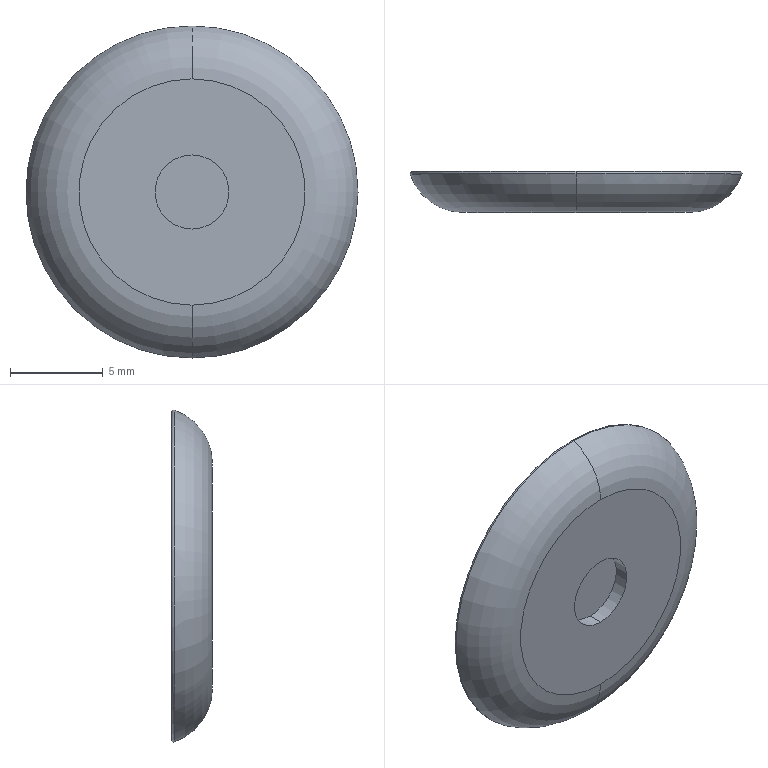Part | SolidWorks | features Revolution 1 | 1 solid | 23 faces | box 17.931 x 2.2 x 17.931 mm | volume 454.739 mm3 | torus 12 | cylinder 6 | plane 5 | commonest cylinder face diameters 4 x2 15.9 x2 16.5 x2
STEP:
#1=CARTESIAN_POINT('',(0.,1.669,-8.961));
#2=VERTEX_POINT('',#1);
#3=CARTESIAN_POINT('',(0.,1.669,8.961));
#4=VERTEX_POINT('',#3);
#5=CARTESIAN_POINT('',(0.,1.669,0.));
#6=DIRECTION('',(0.,-1.,0.));
#7=DIRECTION('',(0.,0.,-1.));
#8=AXIS2_PLACEMENT_3D('',#5,#6,#7);
#9=CIRCLE('',#8,8.961);
#10=EDGE_CURVE('',#2,#4,#9,.T.);
#11=ORIENTED_EDGE('',*,*,#10,.T.);
#12=CARTESIAN_POINT('',(0.,-0.4,6.109));
#13=VERTEX_POINT('',#12);
#14=CARTESIAN_POINT('',(0.,2.6,6.109));
#15=DIRECTION('',(1.,0.,0.));
#16=DIRECTION('',(0.,0.,-1.));
#17=AXIS2_PLACEMENT_3D('',#14,#15,#16);
#18=CIRCLE('',#17,3.);
#19=EDGE_CURVE('',#4,#13,#18,.T.);
#20=ORIENTED_EDGE('',*,*,#19,.T.);
#21=CARTESIAN_POINT('',(0.,-0.4,-6.109));
#22=VERTEX_POINT('',#21);
#23=CARTESIAN_POINT('',(0.,-0.4,0.));
#24=DIRECTION('',(0.,-1.,0.));
#25=DIRECTION('',(0.,0.,-1.));
#26=AXIS2_PLACEMENT_3D('',#23,#24,#25);
#27=CIRCLE('',#26,6.109);
#28=EDGE_CURVE('',#22,#13,#27,.T.);
#29=ORIENTED_EDGE('',*,*,#28,.F.);
#30=CARTESIAN_POINT('',(0.,2.6,-6.109));
#31=DIRECTION('',(-1.,0.,0.));
#32=DIRECTION('',(0.,0.,1.));
#33=AXIS2_PLACEMENT_3D('',#30,#31,#32);
#34=CIRCLE('',#33,3.);
#35=EDGE_CURVE('',#2,#22,#34,.T.);
#36=ORIENTED_EDGE('',*,*,#35,.F.);
#37=EDGE_LOOP('',(#11,#20,#29,#36));
#38=FACE_OUTER_BOUND('',#37,.T.);
#39=CARTESIAN_POINT('',(0.,2.6,0.));
#40=DIRECTION('',(0.,-1.,0.));
#41=DIRECTION('',(0.,0.,-1.));
#42=AXIS2_PLACEMENT_3D('',#39,#40,#41);
#43=TOROIDAL_SURFACE('',#42,6.109,3.);
#44=ADVANCED_FACE('',(#38),#43,.T.);
#45=CARTESIAN_POINT('',(0.,0.4,2.));
#46=VERTEX_POINT('',#45);
#47=CARTESIAN_POINT('',(0.,0.4,-2.));
#48=VERTEX_POINT('',#47);
#49=CARTESIAN_POINT('',(0.,0.4,0.));
#50=DIRECTION('',(0.,-1.,0.));
#51=DIRECTION('',(0.,0.,-1.));
#52=AXIS2_PLACEMENT_3D('',#49,#50,#51);
#53=CIRCLE('',#52,2.);
#54=EDGE_CURVE('',#46,#48,#53,.T.);
#55=ORIENTED_EDGE('',*,*,#54,.F.);
#56=CARTESIAN_POINT('',(0.,-0.4,2.));
#57=VERTEX_POINT('',#56);
#58=CARTESIAN_POINT('',(0.,0.,2.));
#59=DIRECTION('',(0.,-1.,0.));
#60=VECTOR('',#59,1000.);
#61=LINE('',#58,#60);
#62=EDGE_CURVE('',#46,#57,#61,.T.);
#63=ORIENTED_EDGE('',*,*,#62,.T.);
#64=CARTESIAN_POINT('',(0.,-0.4,-2.));
#65=VERTEX_POINT('',#64);
#66=CARTESIAN_POINT('',(0.,-0.4,0.));
#67=DIRECTION('',(0.,-1.,0.));
#68=DIRECTION('',(0.,0.,-1.));
#69=AXIS2_PLACEMENT_3D('',#66,#67,#68);
#70=CIRCLE('',#69,2.);
#71=EDGE_CURVE('',#57,#65,#70,.T.);
#72=ORIENTED_EDGE('',*,*,#71,.T.);
#73=CARTESIAN_POINT('',(0.,0.,-2.));
#74=DIRECTION('',(0.,-1.,0.));
#75=VECTOR('',#74,1000.);
#76=LINE('',#73,#75);
#77=EDGE_CURVE('',#48,#65,#76,.T.);
#78=ORIENTED_EDGE('',*,*,#77,.F.);
#79=EDGE_LOOP('',(#55,#63,#72,#78));
#80=FACE_OUTER_BOUND('',#79,.T.);
#81=CARTESIAN_POINT('',(0.,0.,0.));
#82=DIRECTION('',(0.,-1.,0.));
#83=DIRECTION('',(0.,0.,-1.));
#84=AXIS2_PLACEMENT_3D('',#81,#82,#83);
#85=CYLINDRICAL_SURFACE('',#84,2.);
#86=ADVANCED_FACE('',(#80),#85,.F.);
#87=CARTESIAN_POINT('',(0.,1.8,-7.85));
#88=VERTEX_POINT('',#87);
#89=CARTESIAN_POINT('',(0.,1.8,7.85));
#90=VERTEX_POINT('',#89);
#91=CARTESIAN_POINT('',(0.,1.8,0.));
#92=DIRECTION('',(0.,-1.,0.));
#93=DIRECTION('',(0.,0.,-1.));
#94=AXIS2_PLACEMENT_3D('',#91,#92,#93);
#95=CIRCLE('',#94,7.85);
#96=EDGE_CURVE('',#88,#90,#95,.T.);
#97=ORIENTED_EDGE('',*,*,#96,.T.);
#98=CARTESIAN_POINT('',(0.,1.7,7.95));
#99=VERTEX_POINT('',#98);
#100=CARTESIAN_POINT('',(0.,1.7,7.85));
#101=DIRECTION('',(1.,0.,0.));
#102=DIRECTION('',(0.,0.,-1.));
#103=AXIS2_PLACEMENT_3D('',#100,#101,#102);
#104=CIRCLE('',#103,0.1);
#105=EDGE_CURVE('',#90,#99,#104,.T.);
#106=ORIENTED_EDGE('',*,*,#105,.T.);
#107=CARTESIAN_POINT('',(0.,1.7,-7.95));
#108=VERTEX_POINT('',#107);
#109=CARTESIAN_POINT('',(0.,1.7,0.));
#110=DIRECTION('',(0.,-1.,0.));
#111=DIRECTION('',(0.,0.,-1.));
#112=AXIS2_PLACEMENT_3D('',#109,#110,#111);
#113=CIRCLE('',#112,7.95);
#114=EDGE_CURVE('',#108,#99,#113,.T.);
#115=ORIENTED_EDGE('',*,*,#114,.F.);
#116=CARTESIAN_POINT('',(0.,1.7,-7.85));
#117=DIRECTION('',(-1.,0.,0.));
#118=DIRECTION('',(0.,0.,1.));
#119=AXIS2_PLACEMENT_3D('',#116,#117,#118);
#120=CIRCLE('',#119,0.1);
#121=EDGE_CURVE('',#88,#108,#120,.T.);
#122=ORIENTED_EDGE('',*,*,#121,.F.);
#123=EDGE_LOOP('',(#97,#106,#115,#122));
#124=FACE_OUTER_BOUND('',#123,.T.);
#125=CARTESIAN_POINT('',(0.,1.7,0.));
#126=DIRECTION('',(0.,-1.,0.));
#127=DIRECTION('',(0.,0.,-1.));
#128=AXIS2_PLACEMENT_3D('',#125,#126,#127);
#129=TOROIDAL_SURFACE('',#128,7.85,0.1);
#130=ADVANCED_FACE('',(#124),#129,.T.);
#131=ORIENTED_EDGE('',*,*,#114,.T.);
#132=CARTESIAN_POINT('',(0.,1.4,7.95));
#133=VERTEX_POINT('',#132);
#134=CARTESIAN_POINT('',(0.,0.,7.95));
#135=DIRECTION('',(0.,-1.,0.));
#136=VECTOR('',#135,1000.);
#137=LINE('',#134,#136);
#138=EDGE_CURVE('',#99,#133,#137,.T.);
#139=ORIENTED_EDGE('',*,*,#138,.T.);
#140=CARTESIAN_POINT('',(0.,1.4,-7.95));
#141=VERTEX_POINT('',#140);
#142=CARTESIAN_POINT('',(0.,1.4,0.));
#143=DIRECTION('',(0.,-1.,0.));
#144=DIRECTION('',(0.,0.,-1.));
#145=AXIS2_PLACEMENT_3D('',#142,#143,#144);
#146=CIRCLE('',#145,7.95);
#147=EDGE_CURVE('',#141,#133,#146,.T.);
#148=ORIENTED_EDGE('',*,*,#147,.F.);
#149=CARTESIAN_POINT('',(0.,0.,-7.95));
#150=DIRECTION('',(0.,-1.,0.));
#151=VECTOR('',#150,1000.);
#152=LINE('',#149,#151);
#153=EDGE_CURVE('',#108,#141,#152,.T.);
#154=ORIENTED_EDGE('',*,*,#153,.F.);
#155=EDGE_LOOP('',(#131,#139,#148,#154));
#156=FACE_OUTER_BOUND('',#155,.T.);
#157=CARTESIAN_POINT('',(0.,0.,0.));
#158=DIRECTION('',(0.,-1.,0.));
#159=DIRECTION('',(0.,0.,-1.));
#160=AXIS2_PLACEMENT_3D('',#157,#158,#159);
#161=CYLINDRICAL_SURFACE('',#160,7.95);
#162=ADVANCED_FACE('',(#156),#161,.T.);
#163=CARTESIAN_POINT('',(0.,1.3,8.05));
#164=VERTEX_POINT('',#163);
#165=CARTESIAN_POINT('',(0.,1.3,-8.05));
#166=VERTEX_POINT('',#165);
#167=CARTESIAN_POINT('',(0.,1.3,0.));
#168=DIRECTION('',(0.,-1.,0.));
#169=DIRECTION('',(0.,0.,-1.));
#170=AXIS2_PLACEMENT_3D('',#167,#168,#169);
#171=CIRCLE('',#170,8.05);
#172=EDGE_CURVE('',#164,#166,#171,.T.);
#173=ORIENTED_EDGE('',*,*,#172,.F.);
#174=CARTESIAN_POINT('',(0.,1.4,8.05));
#175=DIRECTION('',(1.,0.,0.));
#176=DIRECTION('',(0.,0.,-1.));
#177=AXIS2_PLACEMENT_3D('',#174,#175,#176);
#178=CIRCLE('',#177,0.1);
#179=EDGE_CURVE('',#164,#133,#178,.T.);
#180=ORIENTED_EDGE('',*,*,#179,.T.);
#181=CARTESIAN_POINT('',(0.,1.4,0.));
#182=DIRECTION('',(0.,-1.,0.));
#183=DIRECTION('',(0.,0.,-1.));
#184=AXIS2_PLACEMENT_3D('',#181,#182,#183);
#185=CIRCLE('',#184,7.95);
#186=EDGE_CURVE('',#133,#141,#185,.T.);
#187=ORIENTED_EDGE('',*,*,#186,.T.);
#188=CARTESIAN_POINT('',(0.,1.4,-8.05));
#189=DIRECTION('',(-1.,0.,0.));
#190=DIRECTION('',(0.,0.,1.));
#191=AXIS2_PLACEMENT_3D('',#188,#189,#190);
#192=CIRCLE('',#191,0.1);
#193=EDGE_CURVE('',#166,#141,#192,.T.);
#194=ORIENTED_EDGE('',*,*,#193,.F.);
#195=EDGE_LOOP('',(#173,#180,#187,#194));
#196=FACE_OUTER_BOUND('',#195,.T.);
#197=CARTESIAN_POINT('',(0.,1.4,0.));
#198=DIRECTION('',(0.,-1.,0.));
#199=DIRECTION('',(0.,0.,-1.));
#200=AXIS2_PLACEMENT_3D('',#197,#198,#199);
#201=TOROIDAL_SURFACE('',#200,8.05,0.1);
#202=ADVANCED_FACE('',(#196),#201,.F.);
#203=CARTESIAN_POINT('',(0.,1.4,8.25));
#204=VERTEX_POINT('',#203);
#205=CARTESIAN_POINT('',(0.,1.4,-8.25));
#206=VERTEX_POINT('',#205);
#207=CARTESIAN_POINT('',(0.,1.4,0.));
#208=DIRECTION('',(0.,-1.,0.));
#209=DIRECTION('',(0.,0.,-1.));
#210=AXIS2_PLACEMENT_3D('',#207,#208,#209);
#211=CIRCLE('',#210,8.25);
#212=EDGE_CURVE('',#204,#206,#211,.T.);
#213=ORIENTED_EDGE('',*,*,#212,.F.);
#214=CARTESIAN_POINT('',(0.,1.3,8.15));
#215=VERTEX_POINT('',#214);
#216=CARTESIAN_POINT('',(0.,1.4,8.15));
#217=DIRECTION('',(1.,0.,0.));
#218=DIRECTION('',(0.,0.,-1.));
#219=AXIS2_PLACEMENT_3D('',#216,#217,#218);
#220=CIRCLE('',#219,0.1);
#221=EDGE_CURVE('',#204,#215,#220,.T.);
#222=ORIENTED_EDGE('',*,*,#221,.T.);
#223=CARTESIAN_POINT('',(0.,1.3,-8.15));
#224=VERTEX_POINT('',#223);
#225=CARTESIAN_POINT('',(0.,1.3,0.));
#226=DIRECTION('',(0.,-1.,0.));
#227=DIRECTION('',(0.,0.,-1.));
#228=AXIS2_PLACEMENT_3D('',#225,#226,#227);
#229=CIRCLE('',#228,8.15);
#230=EDGE_CURVE('',#215,#224,#229,.T.);
#231=ORIENTED_EDGE('',*,*,#230,.T.);
#232=CARTESIAN_POINT('',(0.,1.4,-8.15));
#233=DIRECTION('',(-1.,0.,0.));
#234=DIRECTION('',(0.,0.,1.));
#235=AXIS2_PLACEMENT_3D('',#232,#233,#234);
#236=CIRCLE('',#235,0.1);
#237=EDGE_CURVE('',#206,#224,#236,.T.);
#238=ORIENTED_EDGE('',*,*,#237,.F.);
#239=EDGE_LOOP('',(#213,#222,#231,#238));
#240=FACE_OUTER_BOUND('',#239,.T.);
#241=CARTESIAN_POINT('',(0.,1.4,0.));
#242=DIRECTION('',(0.,-1.,0.));
#243=DIRECTION('',(0.,0.,-1.));
#244=AXIS2_PLACEMENT_3D('',#241,#242,#243);
#245=TOROIDAL_SURFACE('',#244,8.15,0.1);
#246=ADVANCED_FACE('',(#240),#245,.F.);
#247=CARTESIAN_POINT('',(0.,1.7,8.25));
#248=VERTEX_POINT('',#247);
#249=CARTESIAN_POINT('',(0.,1.7,-8.25));
#250=VERTEX_POINT('',#249);
#251=CARTESIAN_POINT('',(0.,1.7,0.));
#252=DIRECTION('',(0.,-1.,0.));
#253=DIRECTION('',(0.,0.,-1.));
#254=AXIS2_PLACEMENT_3D('',#251,#252,#253);
#255=CIRCLE('',#254,8.25);
#256=EDGE_CURVE('',#248,#250,#255,.T.);
#257=ORIENTED_EDGE('',*,*,#256,.F.);
#258=CARTESIAN_POINT('',(0.,0.,8.25));
#259=DIRECTION('',(0.,-1.,0.));
#260=VECTOR('',#259,1000.);
#261=LINE('',#258,#260);
#262=EDGE_CURVE('',#248,#204,#261,.T.);
#263=ORIENTED_EDGE('',*,*,#262,.T.);
#264=ORIENTED_EDGE('',*,*,#212,.T.);
#265=CARTESIAN_POINT('',(0.,0.,-8.25));
#266=DIRECTION('',(0.,-1.,0.));
#267=VECTOR('',#266,1000.);
#268=LINE('',#265,#267);
#269=EDGE_CURVE('',#250,#206,#268,.T.);
#270=ORIENTED_EDGE('',*,*,#269,.F.);
#271=EDGE_LOOP('',(#257,#263,#264,#270));
#272=FACE_OUTER_BOUND('',#271,.T.);
#273=CARTESIAN_POINT('',(0.,0.,0.));
#274=DIRECTION('',(0.,-1.,0.));
#275=DIRECTION('',(0.,0.,-1.));
#276=AXIS2_PLACEMENT_3D('',#273,#274,#275);
#277=CYLINDRICAL_SURFACE('',#276,8.25);
#278=ADVANCED_FACE('',(#272),#277,.F.);
#279=CARTESIAN_POINT('',(0.,1.7,0.));
#280=DIRECTION('',(0.,-1.,0.));
#281=DIRECTION('',(0.,0.,-1.));
#282=AXIS2_PLACEMENT_3D('',#279,#280,#281);
#283=CIRCLE('',#282,8.25);
#284=EDGE_CURVE('',#250,#248,#283,.T.);
#285=ORIENTED_EDGE('',*,*,#284,.T.);
#286=CARTESIAN_POINT('',(0.,1.8,8.35));
#287=VERTEX_POINT('',#286);
#288=CARTESIAN_POINT('',(0.,1.7,8.35));
#289=DIRECTION('',(1.,0.,0.));
#290=DIRECTION('',(0.,0.,-1.));
#291=AXIS2_PLACEMENT_3D('',#288,#289,#290);
#292=CIRCLE('',#291,0.1);
#293=EDGE_CURVE('',#248,#287,#292,.T.);
#294=ORIENTED_EDGE('',*,*,#293,.T.);
#295=CARTESIAN_POINT('',(0.,1.8,-8.35));
#296=VERTEX_POINT('',#295);
#297=CARTESIAN_POINT('',(0.,1.8,0.));
#298=DIRECTION('',(0.,-1.,0.));
#299=DIRECTION('',(0.,0.,-1.));
#300=AXIS2_PLACEMENT_3D('',#297,#298,#299);
#301=CIRCLE('',#300,8.35);
#302=EDGE_CURVE('',#296,#287,#301,.T.);
#303=ORIENTED_EDGE('',*,*,#302,.F.);
#304=CARTESIAN_POINT('',(0.,1.7,-8.35));
#305=DIRECTION('',(-1.,0.,0.));
#306=DIRECTION('',(0.,0.,1.));
#307=AXIS2_PLACEMENT_3D('',#304,#305,#306);
#308=CIRCLE('',#307,0.1);
#309=EDGE_CURVE('',#250,#296,#308,.T.);
#310=ORIENTED_EDGE('',*,*,#309,.F.);
#311=EDGE_LOOP('',(#285,#294,#303,#310));
#312=FACE_OUTER_BOUND('',#311,.T.);
#313=CARTESIAN_POINT('',(0.,1.7,0.));
#314=DIRECTION('',(0.,-1.,0.));
#315=DIRECTION('',(0.,0.,-1.));
#316=AXIS2_PLACEMENT_3D('',#313,#314,#315);
#317=TOROIDAL_SURFACE('',#316,8.35,0.1);
#318=ADVANCED_FACE('',(#312),#317,.T.);
#319=CARTESIAN_POINT('',(0.,1.8,-8.865));
#320=VERTEX_POINT('',#319);
#321=CARTESIAN_POINT('',(0.,1.8,8.865));
#322=VERTEX_POINT('',#321);
#323=CARTESIAN_POINT('',(0.,1.8,0.));
#324=DIRECTION('',(0.,-1.,0.));
#325=DIRECTION('',(0.,0.,-1.));
#326=AXIS2_PLACEMENT_3D('',#323,#324,#325);
#327=CIRCLE('',#326,8.865);
#328=EDGE_CURVE('',#320,#322,#327,.T.);
#329=ORIENTED_EDGE('',*,*,#328,.T.);
#330=CARTESIAN_POINT('',(0.,1.7,8.865));
#331=DIRECTION('',(1.,0.,0.));
#332=DIRECTION('',(0.,0.,-1.));
#333=AXIS2_PLACEMENT_3D('',#330,#331,#332);
#334=CIRCLE('',#333,0.1);
#335=EDGE_CURVE('',#322,#4,#334,.T.);
#336=ORIENTED_EDGE('',*,*,#335,.T.);
#337=ORIENTED_EDGE('',*,*,#10,.F.);
#338=CARTESIAN_POINT('',(0.,1.7,-8.865));
#339=DIRECTION('',(-1.,0.,0.));
#340=DIRECTION('',(0.,0.,1.));
#341=AXIS2_PLACEMENT_3D('',#338,#339,#340);
#342=CIRCLE('',#341,0.1);
#343=EDGE_CURVE('',#320,#2,#342,.T.);
#344=ORIENTED_EDGE('',*,*,#343,.F.);
#345=EDGE_LOOP('',(#329,#336,#337,#344));
#346=FACE_OUTER_BOUND('',#345,.T.);
#347=CARTESIAN_POINT('',(0.,1.7,0.));
#348=DIRECTION('',(0.,-1.,0.));
#349=DIRECTION('',(0.,0.,-1.));
#350=AXIS2_PLACEMENT_3D('',#347,#348,#349);
#351=TOROIDAL_SURFACE('',#350,8.865,0.1);
#352=ADVANCED_FACE('',(#346),#351,.T.);
#353=ORIENTED_EDGE('',*,*,#335,.F.);
#354=CARTESIAN_POINT('',(0.,1.8,0.));
#355=DIRECTION('',(0.,-1.,0.));
#356=DIRECTION('',(0.,0.,-1.));
#357=AXIS2_PLACEMENT_3D('',#354,#355,#356);
#358=CIRCLE('',#357,8.865);
#359=EDGE_CURVE('',#322,#320,#358,.T.);
#360=ORIENTED_EDGE('',*,*,#359,.T.);
#361=ORIENTED_EDGE('',*,*,#343,.T.);
#362=CARTESIAN_POINT('',(0.,1.669,0.));
#363=DIRECTION('',(0.,-1.,0.));
#364=DIRECTION('',(0.,0.,-1.));
#365=AXIS2_PLACEMENT_3D('',#362,#363,#364);
#366=CIRCLE('',#365,8.961);
#367=EDGE_CURVE('',#4,#2,#366,.T.);
#368=ORIENTED_EDGE('',*,*,#367,.F.);
#369=EDGE_LOOP('',(#353,#360,#361,#368));
#370=FACE_OUTER_BOUND('',#369,.T.);
#371=CARTESIAN_POINT('',(0.,1.7,0.));
#372=DIRECTION('',(0.,-1.,0.));
#373=DIRECTION('',(0.,0.,-1.));
#374=AXIS2_PLACEMENT_3D('',#371,#372,#373);
#375=TOROIDAL_SURFACE('',#374,8.865,0.1);
#376=ADVANCED_FACE('',(#370),#375,.T.);
#377=ORIENTED_EDGE('',*,*,#328,.F.);
#378=ORIENTED_EDGE('',*,*,#359,.F.);
#379=EDGE_LOOP('',(#377,#378));
#380=FACE_OUTER_BOUND('',#379,.T.);
#381=ORIENTED_EDGE('',*,*,#302,.T.);
#382=CARTESIAN_POINT('',(0.,1.8,0.));
#383=DIRECTION('',(0.,-1.,0.));
#384=DIRECTION('',(0.,0.,-1.));
#385=AXIS2_PLACEMENT_3D('',#382,#383,#384);
#386=CIRCLE('',#385,8.35);
#387=EDGE_CURVE('',#287,#296,#386,.T.);
#388=ORIENTED_EDGE('',*,*,#387,.T.);
#389=EDGE_LOOP('',(#381,#388));
#390=FACE_BOUND('',#389,.T.);
#391=CARTESIAN_POINT('',(-8.865,1.8,0.));
#392=DIRECTION('',(0.,-1.,0.));
#393=DIRECTION('',(0.,0.,-1.));
#394=AXIS2_PLACEMENT_3D('',#391,#392,#393);
#395=PLANE('',#394);
#396=ADVANCED_FACE('',(#380,#390),#395,.F.);
#397=ORIENTED_EDGE('',*,*,#293,.F.);
#398=ORIENTED_EDGE('',*,*,#256,.T.);
#399=ORIENTED_EDGE('',*,*,#309,.T.);
#400=ORIENTED_EDGE('',*,*,#387,.F.);
#401=EDGE_LOOP('',(#397,#398,#399,#400));
#402=FACE_OUTER_BOUND('',#401,.T.);
#403=CARTESIAN_POINT('',(0.,1.7,0.));
#404=DIRECTION('',(0.,-1.,0.));
#405=DIRECTION('',(0.,0.,-1.));
#406=AXIS2_PLACEMENT_3D('',#403,#404,#405);
#407=TOROIDAL_SURFACE('',#406,8.35,0.1);
#408=ADVANCED_FACE('',(#402),#407,.T.);
#409=ORIENTED_EDGE('',*,*,#262,.F.);
#410=ORIENTED_EDGE('',*,*,#284,.F.);
#411=ORIENTED_EDGE('',*,*,#269,.T.);
#412=CARTESIAN_POINT('',(0.,1.4,0.));
#413=DIRECTION('',(0.,-1.,0.));
#414=DIRECTION('',(0.,0.,-1.));
#415=AXIS2_PLACEMENT_3D('',#412,#413,#414);
#416=CIRCLE('',#415,8.25);
#417=EDGE_CURVE('',#206,#204,#416,.T.);
#418=ORIENTED_EDGE('',*,*,#417,.T.);
#419=EDGE_LOOP('',(#409,#410,#411,#418));
#420=FACE_OUTER_BOUND('',#419,.T.);
#421=CARTESIAN_POINT('',(0.,0.,0.));
#422=DIRECTION('',(0.,-1.,0.));
#423=DIRECTION('',(0.,0.,-1.));
#424=AXIS2_PLACEMENT_3D('',#421,#422,#423);
#425=CYLINDRICAL_SURFACE('',#424,8.25);
#426=ADVANCED_FACE('',(#420),#425,.F.);
#427=ORIENTED_EDGE('',*,*,#221,.F.);
#428=ORIENTED_EDGE('',*,*,#417,.F.);
#429=ORIENTED_EDGE('',*,*,#237,.T.);
#430=CARTESIAN_POINT('',(0.,1.3,0.));
#431=DIRECTION('',(0.,-1.,0.));
#432=DIRECTION('',(0.,0.,-1.));
#433=AXIS2_PLACEMENT_3D('',#430,#431,#432);
#434=CIRCLE('',#433,8.15);
#435=EDGE_CURVE('',#224,#215,#434,.T.);
#436=ORIENTED_EDGE('',*,*,#435,.T.);
#437=EDGE_LOOP('',(#427,#428,#429,#436));
#438=FACE_OUTER_BOUND('',#437,.T.);
#439=CARTESIAN_POINT('',(0.,1.4,0.));
#440=DIRECTION('',(0.,-1.,0.));
#441=DIRECTION('',(0.,0.,-1.));
#442=AXIS2_PLACEMENT_3D('',#439,#440,#441);
#443=TOROIDAL_SURFACE('',#442,8.15,0.1);
#444=ADVANCED_FACE('',(#438),#443,.F.);
#445=ORIENTED_EDGE('',*,*,#435,.F.);
#446=ORIENTED_EDGE('',*,*,#230,.F.);
#447=EDGE_LOOP('',(#445,#446));
#448=FACE_OUTER_BOUND('',#447,.T.);
#449=CARTESIAN_POINT('',(0.,1.3,0.));
#450=DIRECTION('',(0.,-1.,0.));
#451=DIRECTION('',(0.,0.,-1.));
#452=AXIS2_PLACEMENT_3D('',#449,#450,#451);
#453=CIRCLE('',#452,8.05);
#454=EDGE_CURVE('',#166,#164,#453,.T.);
#455=ORIENTED_EDGE('',*,*,#454,.T.);
#456=ORIENTED_EDGE('',*,*,#172,.T.);
#457=EDGE_LOOP('',(#455,#456));
#458=FACE_BOUND('',#457,.T.);
#459=CARTESIAN_POINT('',(-8.15,1.3,0.));
#460=DIRECTION('',(0.,-1.,0.));
#461=DIRECTION('',(0.,0.,-1.));
#462=AXIS2_PLACEMENT_3D('',#459,#460,#461);
#463=PLANE('',#462);
#464=ADVANCED_FACE('',(#448,#458),#463,.F.);
#465=ORIENTED_EDGE('',*,*,#179,.F.);
#466=ORIENTED_EDGE('',*,*,#454,.F.);
#467=ORIENTED_EDGE('',*,*,#193,.T.);
#468=ORIENTED_EDGE('',*,*,#147,.T.);
#469=EDGE_LOOP('',(#465,#466,#467,#468));
#470=FACE_OUTER_BOUND('',#469,.T.);
#471=CARTESIAN_POINT('',(0.,1.4,0.));
#472=DIRECTION('',(0.,-1.,0.));
#473=DIRECTION('',(0.,0.,-1.));
#474=AXIS2_PLACEMENT_3D('',#471,#472,#473);
#475=TOROIDAL_SURFACE('',#474,8.05,0.1);
#476=ADVANCED_FACE('',(#470),#475,.F.);
#477=ORIENTED_EDGE('',*,*,#138,.F.);
#478=CARTESIAN_POINT('',(0.,1.7,0.));
#479=DIRECTION('',(0.,-1.,0.));
#480=DIRECTION('',(0.,0.,-1.));
#481=AXIS2_PLACEMENT_3D('',#478,#479,#480);
#482=CIRCLE('',#481,7.95);
#483=EDGE_CURVE('',#99,#108,#482,.T.);
#484=ORIENTED_EDGE('',*,*,#483,.T.);
#485=ORIENTED_EDGE('',*,*,#153,.T.);
#486=ORIENTED_EDGE('',*,*,#186,.F.);
#487=EDGE_LOOP('',(#477,#484,#485,#486));
#488=FACE_OUTER_BOUND('',#487,.T.);
#489=CARTESIAN_POINT('',(0.,0.,0.));
#490=DIRECTION('',(0.,-1.,0.));
#491=DIRECTION('',(0.,0.,-1.));
#492=AXIS2_PLACEMENT_3D('',#489,#490,#491);
#493=CYLINDRICAL_SURFACE('',#492,7.95);
#494=ADVANCED_FACE('',(#488),#493,.T.);
#495=ORIENTED_EDGE('',*,*,#105,.F.);
#496=CARTESIAN_POINT('',(0.,1.8,0.));
#497=DIRECTION('',(0.,-1.,0.));
#498=DIRECTION('',(0.,0.,-1.));
#499=AXIS2_PLACEMENT_3D('',#496,#497,#498);
#500=CIRCLE('',#499,7.85);
#501=EDGE_CURVE('',#90,#88,#500,.T.);
#502=ORIENTED_EDGE('',*,*,#501,.T.);
#503=ORIENTED_EDGE('',*,*,#121,.T.);
#504=ORIENTED_EDGE('',*,*,#483,.F.);
#505=EDGE_LOOP('',(#495,#502,#503,#504));
#506=FACE_OUTER_BOUND('',#505,.T.);
#507=CARTESIAN_POINT('',(0.,1.7,0.));
#508=DIRECTION('',(0.,-1.,0.));
#509=DIRECTION('',(0.,0.,-1.));
#510=AXIS2_PLACEMENT_3D('',#507,#508,#509);
#511=TOROIDAL_SURFACE('',#510,7.85,0.1);
#512=ADVANCED_FACE('',(#506),#511,.T.);
#513=ORIENTED_EDGE('',*,*,#96,.F.);
#514=ORIENTED_EDGE('',*,*,#501,.F.);
#515=EDGE_LOOP('',(#513,#514));
#516=FACE_OUTER_BOUND('',#515,.T.);
#517=CARTESIAN_POINT('',(-7.85,1.8,0.));
#518=DIRECTION('',(0.,-1.,0.));
#519=DIRECTION('',(0.,0.,-1.));
#520=AXIS2_PLACEMENT_3D('',#517,#518,#519);
#521=PLANE('',#520);
#522=ADVANCED_FACE('',(#516),#521,.F.);
#523=CARTESIAN_POINT('',(0.,0.4,0.));
#524=DIRECTION('',(0.,-1.,0.));
#525=DIRECTION('',(0.,0.,-1.));
#526=AXIS2_PLACEMENT_3D('',#523,#524,#525);
#527=CIRCLE('',#526,2.);
#528=EDGE_CURVE('',#48,#46,#527,.T.);
#529=ORIENTED_EDGE('',*,*,#528,.T.);
#530=ORIENTED_EDGE('',*,*,#54,.T.);
#531=EDGE_LOOP('',(#529,#530));
#532=FACE_OUTER_BOUND('',#531,.T.);
#533=CARTESIAN_POINT('',(0.,0.4,0.));
#534=DIRECTION('',(0.,1.,0.));
#535=DIRECTION('',(0.,0.,1.));
#536=AXIS2_PLACEMENT_3D('',#533,#534,#535);
#537=PLANE('',#536);
#538=ADVANCED_FACE('',(#532),#537,.F.);
#539=ORIENTED_EDGE('',*,*,#62,.F.);
#540=ORIENTED_EDGE('',*,*,#528,.F.);
#541=ORIENTED_EDGE('',*,*,#77,.T.);
#542=CARTESIAN_POINT('',(0.,-0.4,0.));
#543=DIRECTION('',(0.,-1.,0.));
#544=DIRECTION('',(0.,0.,-1.));
#545=AXIS2_PLACEMENT_3D('',#542,#543,#544);
#546=CIRCLE('',#545,2.);
#547=EDGE_CURVE('',#65,#57,#546,.T.);
#548=ORIENTED_EDGE('',*,*,#547,.T.);
#549=EDGE_LOOP('',(#539,#540,#541,#548));
#550=FACE_OUTER_BOUND('',#549,.T.);
#551=CARTESIAN_POINT('',(0.,0.,0.));
#552=DIRECTION('',(0.,-1.,0.));
#553=DIRECTION('',(0.,0.,-1.));
#554=AXIS2_PLACEMENT_3D('',#551,#552,#553);
#555=CYLINDRICAL_SURFACE('',#554,2.);
#556=ADVANCED_FACE('',(#550),#555,.F.);
#557=ORIENTED_EDGE('',*,*,#547,.F.);
#558=ORIENTED_EDGE('',*,*,#71,.F.);
#559=EDGE_LOOP('',(#557,#558));
#560=FACE_BOUND('',#559,.T.);
#561=ORIENTED_EDGE('',*,*,#28,.T.);
#562=CARTESIAN_POINT('',(0.,-0.4,0.));
#563=DIRECTION('',(0.,-1.,0.));
#564=DIRECTION('',(0.,0.,-1.));
#565=AXIS2_PLACEMENT_3D('',#562,#563,#564);
#566=CIRCLE('',#565,6.109);
#567=EDGE_CURVE('',#13,#22,#566,.T.);
#568=ORIENTED_EDGE('',*,*,#567,.T.);
#569=EDGE_LOOP('',(#561,#568));
#570=FACE_OUTER_BOUND('',#569,.T.);
#571=CARTESIAN_POINT('',(-2.,-0.4,0.));
#572=DIRECTION('',(0.,1.,0.));
#573=DIRECTION('',(0.,0.,1.));
#574=AXIS2_PLACEMENT_3D('',#571,#572,#573);
#575=PLANE('',#574);
#576=ADVANCED_FACE('',(#560,#570),#575,.F.);
#577=ORIENTED_EDGE('',*,*,#19,.F.);
#578=ORIENTED_EDGE('',*,*,#367,.T.);
#579=ORIENTED_EDGE('',*,*,#35,.T.);
#580=ORIENTED_EDGE('',*,*,#567,.F.);
#581=EDGE_LOOP('',(#577,#578,#579,#580));
#582=FACE_OUTER_BOUND('',#581,.T.);
#583=CARTESIAN_POINT('',(0.,2.6,0.));
#584=DIRECTION('',(0.,-1.,0.));
#585=DIRECTION('',(0.,0.,-1.));
#586=AXIS2_PLACEMENT_3D('',#583,#584,#585);
#587=TOROIDAL_SURFACE('',#586,6.109,3.);
#588=ADVANCED_FACE('',(#582),#587,.T.);
#589=CLOSED_SHELL('',(#44,#86,#130,#162,#202,#246,#278,#318,#352,#376,#396,#408,#426,#444,#464,#476,#494,#512,#522,#538,#556,#576,#588));
#590=MANIFOLD_SOLID_BREP('',#589);
#591=CARTESIAN_POINT('',(0.,0.,0.));
#592=DIRECTION('',(0.,0.,1.));
#593=DIRECTION('',(1.,0.,0.));
#594=AXIS2_PLACEMENT_3D('',#591,#592,#593);
#595=(LENGTH_UNIT()NAMED_UNIT(*)SI_UNIT(.MILLI.,.METRE.));
#596=UNCERTAINTY_MEASURE_WITH_UNIT(LENGTH_MEASURE(0.00001),#595,'','');
#597=(NAMED_UNIT(*)PLANE_ANGLE_UNIT()SI_UNIT($,.RADIAN.));
#598=(NAMED_UNIT(*)SI_UNIT($,.STERADIAN.)SOLID_ANGLE_UNIT());
#599=(GEOMETRIC_REPRESENTATION_CONTEXT(3)GLOBAL_UNCERTAINTY_ASSIGNED_CONTEXT((#596))GLOBAL_UNIT_ASSIGNED_CONTEXT((#595,#597,#598))REPRESENTATION_CONTEXT('',''));
#600=ADVANCED_BREP_SHAPE_REPRESENTATION('',(#590,#594),#599);